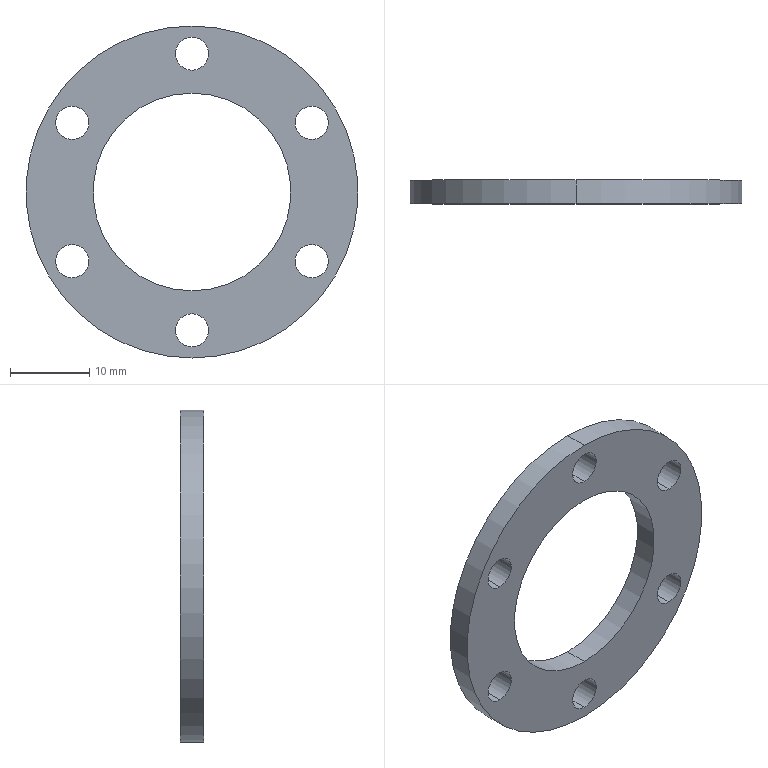Part | SolidWorks | features Extrusion 1 | 1 solid | 18 faces | box 42 x 3 x 42 mm | volume 2434 mm3 | cylinder 16 | plane 2 | commonest cylinder face diameters 4.2 x12 25 x2 42 x2
STEP:
#1=CARTESIAN_POINT('',(-15.155,3.,-10.85));
#2=VERTEX_POINT('',#1);
#3=CARTESIAN_POINT('',(-15.155,3.,-6.65));
#4=VERTEX_POINT('',#3);
#5=CARTESIAN_POINT('',(-15.155,3.,-8.75));
#6=DIRECTION('',(0.,1.,0.));
#7=DIRECTION('',(0.,0.,1.));
#8=AXIS2_PLACEMENT_3D('',#5,#6,#7);
#9=CIRCLE('',#8,2.1);
#10=EDGE_CURVE('',#2,#4,#9,.T.);
#11=ORIENTED_EDGE('',*,*,#10,.T.);
#12=CARTESIAN_POINT('',(-15.155,0.,-6.65));
#13=VERTEX_POINT('',#12);
#14=CARTESIAN_POINT('',(-15.155,3.,-6.65));
#15=DIRECTION('',(0.,-1.,0.));
#16=VECTOR('',#15,1000.);
#17=LINE('',#14,#16);
#18=EDGE_CURVE('',#4,#13,#17,.T.);
#19=ORIENTED_EDGE('',*,*,#18,.T.);
#20=CARTESIAN_POINT('',(-15.155,0.,-10.85));
#21=VERTEX_POINT('',#20);
#22=CARTESIAN_POINT('',(-15.155,0.,-8.75));
#23=DIRECTION('',(0.,1.,0.));
#24=DIRECTION('',(0.,0.,1.));
#25=AXIS2_PLACEMENT_3D('',#22,#23,#24);
#26=CIRCLE('',#25,2.1);
#27=EDGE_CURVE('',#21,#13,#26,.T.);
#28=ORIENTED_EDGE('',*,*,#27,.F.);
#29=CARTESIAN_POINT('',(-15.155,3.,-10.85));
#30=DIRECTION('',(0.,-1.,0.));
#31=VECTOR('',#30,1000.);
#32=LINE('',#29,#31);
#33=EDGE_CURVE('',#2,#21,#32,.T.);
#34=ORIENTED_EDGE('',*,*,#33,.F.);
#35=EDGE_LOOP('',(#11,#19,#28,#34));
#36=FACE_OUTER_BOUND('',#35,.T.);
#37=CARTESIAN_POINT('',(-15.155,3.,-8.75));
#38=DIRECTION('',(0.,-1.,0.));
#39=DIRECTION('',(0.,0.,-1.));
#40=AXIS2_PLACEMENT_3D('',#37,#38,#39);
#41=CYLINDRICAL_SURFACE('',#40,2.1);
#42=ADVANCED_FACE('',(#36),#41,.F.);
#43=CARTESIAN_POINT('',(-15.155,3.,6.65));
#44=VERTEX_POINT('',#43);
#45=CARTESIAN_POINT('',(-15.155,3.,10.85));
#46=VERTEX_POINT('',#45);
#47=CARTESIAN_POINT('',(-15.155,3.,8.75));
#48=DIRECTION('',(0.,1.,0.));
#49=DIRECTION('',(0.,0.,1.));
#50=AXIS2_PLACEMENT_3D('',#47,#48,#49);
#51=CIRCLE('',#50,2.1);
#52=EDGE_CURVE('',#44,#46,#51,.T.);
#53=ORIENTED_EDGE('',*,*,#52,.T.);
#54=CARTESIAN_POINT('',(-15.155,0.,10.85));
#55=VERTEX_POINT('',#54);
#56=CARTESIAN_POINT('',(-15.155,3.,10.85));
#57=DIRECTION('',(0.,-1.,0.));
#58=VECTOR('',#57,1000.);
#59=LINE('',#56,#58);
#60=EDGE_CURVE('',#46,#55,#59,.T.);
#61=ORIENTED_EDGE('',*,*,#60,.T.);
#62=CARTESIAN_POINT('',(-15.155,0.,6.65));
#63=VERTEX_POINT('',#62);
#64=CARTESIAN_POINT('',(-15.155,0.,8.75));
#65=DIRECTION('',(0.,1.,0.));
#66=DIRECTION('',(0.,0.,1.));
#67=AXIS2_PLACEMENT_3D('',#64,#65,#66);
#68=CIRCLE('',#67,2.1);
#69=EDGE_CURVE('',#63,#55,#68,.T.);
#70=ORIENTED_EDGE('',*,*,#69,.F.);
#71=CARTESIAN_POINT('',(-15.155,3.,6.65));
#72=DIRECTION('',(0.,-1.,0.));
#73=VECTOR('',#72,1000.);
#74=LINE('',#71,#73);
#75=EDGE_CURVE('',#44,#63,#74,.T.);
#76=ORIENTED_EDGE('',*,*,#75,.F.);
#77=EDGE_LOOP('',(#53,#61,#70,#76));
#78=FACE_OUTER_BOUND('',#77,.T.);
#79=CARTESIAN_POINT('',(-15.155,3.,8.75));
#80=DIRECTION('',(0.,-1.,0.));
#81=DIRECTION('',(0.,0.,-1.));
#82=AXIS2_PLACEMENT_3D('',#79,#80,#81);
#83=CYLINDRICAL_SURFACE('',#82,2.1);
#84=ADVANCED_FACE('',(#78),#83,.F.);
#85=CARTESIAN_POINT('',(0.,3.,15.4));
#86=VERTEX_POINT('',#85);
#87=CARTESIAN_POINT('',(0.,3.,19.6));
#88=VERTEX_POINT('',#87);
#89=CARTESIAN_POINT('',(0.,3.,17.5));
#90=DIRECTION('',(0.,1.,0.));
#91=DIRECTION('',(0.,0.,1.));
#92=AXIS2_PLACEMENT_3D('',#89,#90,#91);
#93=CIRCLE('',#92,2.1);
#94=EDGE_CURVE('',#86,#88,#93,.T.);
#95=ORIENTED_EDGE('',*,*,#94,.T.);
#96=CARTESIAN_POINT('',(0.,0.,19.6));
#97=VERTEX_POINT('',#96);
#98=CARTESIAN_POINT('',(0.,3.,19.6));
#99=DIRECTION('',(0.,-1.,0.));
#100=VECTOR('',#99,1000.);
#101=LINE('',#98,#100);
#102=EDGE_CURVE('',#88,#97,#101,.T.);
#103=ORIENTED_EDGE('',*,*,#102,.T.);
#104=CARTESIAN_POINT('',(0.,0.,15.4));
#105=VERTEX_POINT('',#104);
#106=CARTESIAN_POINT('',(0.,0.,17.5));
#107=DIRECTION('',(0.,1.,0.));
#108=DIRECTION('',(0.,0.,1.));
#109=AXIS2_PLACEMENT_3D('',#106,#107,#108);
#110=CIRCLE('',#109,2.1);
#111=EDGE_CURVE('',#105,#97,#110,.T.);
#112=ORIENTED_EDGE('',*,*,#111,.F.);
#113=CARTESIAN_POINT('',(0.,3.,15.4));
#114=DIRECTION('',(0.,-1.,0.));
#115=VECTOR('',#114,1000.);
#116=LINE('',#113,#115);
#117=EDGE_CURVE('',#86,#105,#116,.T.);
#118=ORIENTED_EDGE('',*,*,#117,.F.);
#119=EDGE_LOOP('',(#95,#103,#112,#118));
#120=FACE_OUTER_BOUND('',#119,.T.);
#121=CARTESIAN_POINT('',(0.,3.,17.5));
#122=DIRECTION('',(0.,-1.,0.));
#123=DIRECTION('',(0.,0.,-1.));
#124=AXIS2_PLACEMENT_3D('',#121,#122,#123);
#125=CYLINDRICAL_SURFACE('',#124,2.1);
#126=ADVANCED_FACE('',(#120),#125,.F.);
#127=CARTESIAN_POINT('',(15.155,3.,6.65));
#128=VERTEX_POINT('',#127);
#129=CARTESIAN_POINT('',(15.155,3.,10.85));
#130=VERTEX_POINT('',#129);
#131=CARTESIAN_POINT('',(15.155,3.,8.75));
#132=DIRECTION('',(0.,1.,0.));
#133=DIRECTION('',(0.,0.,1.));
#134=AXIS2_PLACEMENT_3D('',#131,#132,#133);
#135=CIRCLE('',#134,2.1);
#136=EDGE_CURVE('',#128,#130,#135,.T.);
#137=ORIENTED_EDGE('',*,*,#136,.T.);
#138=CARTESIAN_POINT('',(15.155,0.,10.85));
#139=VERTEX_POINT('',#138);
#140=CARTESIAN_POINT('',(15.155,3.,10.85));
#141=DIRECTION('',(0.,-1.,0.));
#142=VECTOR('',#141,1000.);
#143=LINE('',#140,#142);
#144=EDGE_CURVE('',#130,#139,#143,.T.);
#145=ORIENTED_EDGE('',*,*,#144,.T.);
#146=CARTESIAN_POINT('',(15.155,0.,6.65));
#147=VERTEX_POINT('',#146);
#148=CARTESIAN_POINT('',(15.155,0.,8.75));
#149=DIRECTION('',(0.,1.,0.));
#150=DIRECTION('',(0.,0.,1.));
#151=AXIS2_PLACEMENT_3D('',#148,#149,#150);
#152=CIRCLE('',#151,2.1);
#153=EDGE_CURVE('',#147,#139,#152,.T.);
#154=ORIENTED_EDGE('',*,*,#153,.F.);
#155=CARTESIAN_POINT('',(15.155,3.,6.65));
#156=DIRECTION('',(0.,-1.,0.));
#157=VECTOR('',#156,1000.);
#158=LINE('',#155,#157);
#159=EDGE_CURVE('',#128,#147,#158,.T.);
#160=ORIENTED_EDGE('',*,*,#159,.F.);
#161=EDGE_LOOP('',(#137,#145,#154,#160));
#162=FACE_OUTER_BOUND('',#161,.T.);
#163=CARTESIAN_POINT('',(15.155,3.,8.75));
#164=DIRECTION('',(0.,-1.,0.));
#165=DIRECTION('',(0.,0.,-1.));
#166=AXIS2_PLACEMENT_3D('',#163,#164,#165);
#167=CYLINDRICAL_SURFACE('',#166,2.1);
#168=ADVANCED_FACE('',(#162),#167,.F.);
#169=CARTESIAN_POINT('',(15.155,3.,-10.85));
#170=VERTEX_POINT('',#169);
#171=CARTESIAN_POINT('',(15.155,3.,-6.65));
#172=VERTEX_POINT('',#171);
#173=CARTESIAN_POINT('',(15.155,3.,-8.75));
#174=DIRECTION('',(0.,1.,0.));
#175=DIRECTION('',(0.,0.,1.));
#176=AXIS2_PLACEMENT_3D('',#173,#174,#175);
#177=CIRCLE('',#176,2.1);
#178=EDGE_CURVE('',#170,#172,#177,.T.);
#179=ORIENTED_EDGE('',*,*,#178,.T.);
#180=CARTESIAN_POINT('',(15.155,0.,-6.65));
#181=VERTEX_POINT('',#180);
#182=CARTESIAN_POINT('',(15.155,3.,-6.65));
#183=DIRECTION('',(0.,-1.,0.));
#184=VECTOR('',#183,1000.);
#185=LINE('',#182,#184);
#186=EDGE_CURVE('',#172,#181,#185,.T.);
#187=ORIENTED_EDGE('',*,*,#186,.T.);
#188=CARTESIAN_POINT('',(15.155,0.,-10.85));
#189=VERTEX_POINT('',#188);
#190=CARTESIAN_POINT('',(15.155,0.,-8.75));
#191=DIRECTION('',(0.,1.,0.));
#192=DIRECTION('',(0.,0.,1.));
#193=AXIS2_PLACEMENT_3D('',#190,#191,#192);
#194=CIRCLE('',#193,2.1);
#195=EDGE_CURVE('',#189,#181,#194,.T.);
#196=ORIENTED_EDGE('',*,*,#195,.F.);
#197=CARTESIAN_POINT('',(15.155,3.,-10.85));
#198=DIRECTION('',(0.,-1.,0.));
#199=VECTOR('',#198,1000.);
#200=LINE('',#197,#199);
#201=EDGE_CURVE('',#170,#189,#200,.T.);
#202=ORIENTED_EDGE('',*,*,#201,.F.);
#203=EDGE_LOOP('',(#179,#187,#196,#202));
#204=FACE_OUTER_BOUND('',#203,.T.);
#205=CARTESIAN_POINT('',(15.155,3.,-8.75));
#206=DIRECTION('',(0.,-1.,0.));
#207=DIRECTION('',(0.,0.,-1.));
#208=AXIS2_PLACEMENT_3D('',#205,#206,#207);
#209=CYLINDRICAL_SURFACE('',#208,2.1);
#210=ADVANCED_FACE('',(#204),#209,.F.);
#211=CARTESIAN_POINT('',(0.,3.,-19.6));
#212=VERTEX_POINT('',#211);
#213=CARTESIAN_POINT('',(0.,3.,-15.4));
#214=VERTEX_POINT('',#213);
#215=CARTESIAN_POINT('',(0.,3.,-17.5));
#216=DIRECTION('',(0.,1.,0.));
#217=DIRECTION('',(0.,0.,1.));
#218=AXIS2_PLACEMENT_3D('',#215,#216,#217);
#219=CIRCLE('',#218,2.1);
#220=EDGE_CURVE('',#212,#214,#219,.T.);
#221=ORIENTED_EDGE('',*,*,#220,.T.);
#222=CARTESIAN_POINT('',(0.,0.,-15.4));
#223=VERTEX_POINT('',#222);
#224=CARTESIAN_POINT('',(0.,3.,-15.4));
#225=DIRECTION('',(0.,-1.,0.));
#226=VECTOR('',#225,1000.);
#227=LINE('',#224,#226);
#228=EDGE_CURVE('',#214,#223,#227,.T.);
#229=ORIENTED_EDGE('',*,*,#228,.T.);
#230=CARTESIAN_POINT('',(0.,0.,-19.6));
#231=VERTEX_POINT('',#230);
#232=CARTESIAN_POINT('',(0.,0.,-17.5));
#233=DIRECTION('',(0.,1.,0.));
#234=DIRECTION('',(0.,0.,1.));
#235=AXIS2_PLACEMENT_3D('',#232,#233,#234);
#236=CIRCLE('',#235,2.1);
#237=EDGE_CURVE('',#231,#223,#236,.T.);
#238=ORIENTED_EDGE('',*,*,#237,.F.);
#239=CARTESIAN_POINT('',(0.,3.,-19.6));
#240=DIRECTION('',(0.,-1.,0.));
#241=VECTOR('',#240,1000.);
#242=LINE('',#239,#241);
#243=EDGE_CURVE('',#212,#231,#242,.T.);
#244=ORIENTED_EDGE('',*,*,#243,.F.);
#245=EDGE_LOOP('',(#221,#229,#238,#244));
#246=FACE_OUTER_BOUND('',#245,.T.);
#247=CARTESIAN_POINT('',(0.,3.,-17.5));
#248=DIRECTION('',(0.,-1.,0.));
#249=DIRECTION('',(0.,0.,-1.));
#250=AXIS2_PLACEMENT_3D('',#247,#248,#249);
#251=CYLINDRICAL_SURFACE('',#250,2.1);
#252=ADVANCED_FACE('',(#246),#251,.F.);
#253=CARTESIAN_POINT('',(0.,3.,-12.5));
#254=VERTEX_POINT('',#253);
#255=CARTESIAN_POINT('',(0.,3.,12.5));
#256=VERTEX_POINT('',#255);
#257=CARTESIAN_POINT('',(0.,3.,0.));
#258=DIRECTION('',(0.,1.,0.));
#259=DIRECTION('',(0.,0.,1.));
#260=AXIS2_PLACEMENT_3D('',#257,#258,#259);
#261=CIRCLE('',#260,12.5);
#262=EDGE_CURVE('',#254,#256,#261,.T.);
#263=ORIENTED_EDGE('',*,*,#262,.T.);
#264=CARTESIAN_POINT('',(0.,0.,12.5));
#265=VERTEX_POINT('',#264);
#266=CARTESIAN_POINT('',(0.,3.,12.5));
#267=DIRECTION('',(0.,-1.,0.));
#268=VECTOR('',#267,1000.);
#269=LINE('',#266,#268);
#270=EDGE_CURVE('',#256,#265,#269,.T.);
#271=ORIENTED_EDGE('',*,*,#270,.T.);
#272=CARTESIAN_POINT('',(0.,0.,-12.5));
#273=VERTEX_POINT('',#272);
#274=CARTESIAN_POINT('',(0.,0.,0.));
#275=DIRECTION('',(0.,1.,0.));
#276=DIRECTION('',(0.,0.,1.));
#277=AXIS2_PLACEMENT_3D('',#274,#275,#276);
#278=CIRCLE('',#277,12.5);
#279=EDGE_CURVE('',#273,#265,#278,.T.);
#280=ORIENTED_EDGE('',*,*,#279,.F.);
#281=CARTESIAN_POINT('',(0.,3.,-12.5));
#282=DIRECTION('',(0.,-1.,0.));
#283=VECTOR('',#282,1000.);
#284=LINE('',#281,#283);
#285=EDGE_CURVE('',#254,#273,#284,.T.);
#286=ORIENTED_EDGE('',*,*,#285,.F.);
#287=EDGE_LOOP('',(#263,#271,#280,#286));
#288=FACE_OUTER_BOUND('',#287,.T.);
#289=CARTESIAN_POINT('',(0.,3.,0.));
#290=DIRECTION('',(0.,-1.,0.));
#291=DIRECTION('',(0.,0.,-1.));
#292=AXIS2_PLACEMENT_3D('',#289,#290,#291);
#293=CYLINDRICAL_SURFACE('',#292,12.5);
#294=ADVANCED_FACE('',(#288),#293,.F.);
#295=CARTESIAN_POINT('',(0.,3.,21.));
#296=VERTEX_POINT('',#295);
#297=CARTESIAN_POINT('',(0.,3.,-21.));
#298=VERTEX_POINT('',#297);
#299=CARTESIAN_POINT('',(0.,3.,0.));
#300=DIRECTION('',(0.,1.,0.));
#301=DIRECTION('',(0.,0.,1.));
#302=AXIS2_PLACEMENT_3D('',#299,#300,#301);
#303=CIRCLE('',#302,21.);
#304=EDGE_CURVE('',#296,#298,#303,.T.);
#305=ORIENTED_EDGE('',*,*,#304,.F.);
#306=CARTESIAN_POINT('',(0.,0.,21.));
#307=VERTEX_POINT('',#306);
#308=CARTESIAN_POINT('',(0.,3.,21.));
#309=DIRECTION('',(0.,-1.,0.));
#310=VECTOR('',#309,1000.);
#311=LINE('',#308,#310);
#312=EDGE_CURVE('',#296,#307,#311,.T.);
#313=ORIENTED_EDGE('',*,*,#312,.T.);
#314=CARTESIAN_POINT('',(0.,0.,-21.));
#315=VERTEX_POINT('',#314);
#316=CARTESIAN_POINT('',(0.,0.,0.));
#317=DIRECTION('',(0.,1.,0.));
#318=DIRECTION('',(0.,0.,1.));
#319=AXIS2_PLACEMENT_3D('',#316,#317,#318);
#320=CIRCLE('',#319,21.);
#321=EDGE_CURVE('',#307,#315,#320,.T.);
#322=ORIENTED_EDGE('',*,*,#321,.T.);
#323=CARTESIAN_POINT('',(0.,3.,-21.));
#324=DIRECTION('',(0.,-1.,0.));
#325=VECTOR('',#324,1000.);
#326=LINE('',#323,#325);
#327=EDGE_CURVE('',#298,#315,#326,.T.);
#328=ORIENTED_EDGE('',*,*,#327,.F.);
#329=EDGE_LOOP('',(#305,#313,#322,#328));
#330=FACE_OUTER_BOUND('',#329,.T.);
#331=CARTESIAN_POINT('',(0.,3.,0.));
#332=DIRECTION('',(0.,-1.,0.));
#333=DIRECTION('',(0.,0.,-1.));
#334=AXIS2_PLACEMENT_3D('',#331,#332,#333);
#335=CYLINDRICAL_SURFACE('',#334,21.);
#336=ADVANCED_FACE('',(#330),#335,.T.);
#337=ORIENTED_EDGE('',*,*,#52,.F.);
#338=CARTESIAN_POINT('',(-15.155,3.,8.75));
#339=DIRECTION('',(0.,1.,0.));
#340=DIRECTION('',(0.,0.,1.));
#341=AXIS2_PLACEMENT_3D('',#338,#339,#340);
#342=CIRCLE('',#341,2.1);
#343=EDGE_CURVE('',#46,#44,#342,.T.);
#344=ORIENTED_EDGE('',*,*,#343,.F.);
#345=EDGE_LOOP('',(#337,#344));
#346=FACE_BOUND('',#345,.T.);
#347=ORIENTED_EDGE('',*,*,#136,.F.);
#348=CARTESIAN_POINT('',(15.155,3.,8.75));
#349=DIRECTION('',(0.,1.,0.));
#350=DIRECTION('',(0.,0.,1.));
#351=AXIS2_PLACEMENT_3D('',#348,#349,#350);
#352=CIRCLE('',#351,2.1);
#353=EDGE_CURVE('',#130,#128,#352,.T.);
#354=ORIENTED_EDGE('',*,*,#353,.F.);
#355=EDGE_LOOP('',(#347,#354));
#356=FACE_BOUND('',#355,.T.);
#357=ORIENTED_EDGE('',*,*,#220,.F.);
#358=CARTESIAN_POINT('',(0.,3.,-17.5));
#359=DIRECTION('',(0.,1.,0.));
#360=DIRECTION('',(0.,0.,1.));
#361=AXIS2_PLACEMENT_3D('',#358,#359,#360);
#362=CIRCLE('',#361,2.1);
#363=EDGE_CURVE('',#214,#212,#362,.T.);
#364=ORIENTED_EDGE('',*,*,#363,.F.);
#365=EDGE_LOOP('',(#357,#364));
#366=FACE_BOUND('',#365,.T.);
#367=CARTESIAN_POINT('',(0.,3.,0.));
#368=DIRECTION('',(0.,1.,0.));
#369=DIRECTION('',(0.,0.,1.));
#370=AXIS2_PLACEMENT_3D('',#367,#368,#369);
#371=CIRCLE('',#370,21.);
#372=EDGE_CURVE('',#298,#296,#371,.T.);
#373=ORIENTED_EDGE('',*,*,#372,.T.);
#374=ORIENTED_EDGE('',*,*,#304,.T.);
#375=EDGE_LOOP('',(#373,#374));
#376=FACE_OUTER_BOUND('',#375,.T.);
#377=ORIENTED_EDGE('',*,*,#262,.F.);
#378=CARTESIAN_POINT('',(0.,3.,0.));
#379=DIRECTION('',(0.,1.,0.));
#380=DIRECTION('',(0.,0.,1.));
#381=AXIS2_PLACEMENT_3D('',#378,#379,#380);
#382=CIRCLE('',#381,12.5);
#383=EDGE_CURVE('',#256,#254,#382,.T.);
#384=ORIENTED_EDGE('',*,*,#383,.F.);
#385=EDGE_LOOP('',(#377,#384));
#386=FACE_BOUND('',#385,.T.);
#387=ORIENTED_EDGE('',*,*,#178,.F.);
#388=CARTESIAN_POINT('',(15.155,3.,-8.75));
#389=DIRECTION('',(0.,1.,0.));
#390=DIRECTION('',(0.,0.,1.));
#391=AXIS2_PLACEMENT_3D('',#388,#389,#390);
#392=CIRCLE('',#391,2.1);
#393=EDGE_CURVE('',#172,#170,#392,.T.);
#394=ORIENTED_EDGE('',*,*,#393,.F.);
#395=EDGE_LOOP('',(#387,#394));
#396=FACE_BOUND('',#395,.T.);
#397=ORIENTED_EDGE('',*,*,#94,.F.);
#398=CARTESIAN_POINT('',(0.,3.,17.5));
#399=DIRECTION('',(0.,1.,0.));
#400=DIRECTION('',(0.,0.,1.));
#401=AXIS2_PLACEMENT_3D('',#398,#399,#400);
#402=CIRCLE('',#401,2.1);
#403=EDGE_CURVE('',#88,#86,#402,.T.);
#404=ORIENTED_EDGE('',*,*,#403,.F.);
#405=EDGE_LOOP('',(#397,#404));
#406=FACE_BOUND('',#405,.T.);
#407=ORIENTED_EDGE('',*,*,#10,.F.);
#408=CARTESIAN_POINT('',(-15.155,3.,-8.75));
#409=DIRECTION('',(0.,1.,0.));
#410=DIRECTION('',(0.,0.,1.));
#411=AXIS2_PLACEMENT_3D('',#408,#409,#410);
#412=CIRCLE('',#411,2.1);
#413=EDGE_CURVE('',#4,#2,#412,.T.);
#414=ORIENTED_EDGE('',*,*,#413,.F.);
#415=EDGE_LOOP('',(#407,#414));
#416=FACE_BOUND('',#415,.T.);
#417=CARTESIAN_POINT('',(0.,3.,0.));
#418=DIRECTION('',(0.,1.,0.));
#419=DIRECTION('',(0.,0.,1.));
#420=AXIS2_PLACEMENT_3D('',#417,#418,#419);
#421=PLANE('',#420);
#422=ADVANCED_FACE('',(#346,#356,#366,#376,#386,#396,#406,#416),#421,.T.);
#423=CARTESIAN_POINT('',(0.,0.,0.));
#424=DIRECTION('',(0.,1.,0.));
#425=DIRECTION('',(0.,0.,1.));
#426=AXIS2_PLACEMENT_3D('',#423,#424,#425);
#427=CIRCLE('',#426,21.);
#428=EDGE_CURVE('',#315,#307,#427,.T.);
#429=ORIENTED_EDGE('',*,*,#428,.F.);
#430=ORIENTED_EDGE('',*,*,#321,.F.);
#431=EDGE_LOOP('',(#429,#430));
#432=FACE_OUTER_BOUND('',#431,.T.);
#433=ORIENTED_EDGE('',*,*,#279,.T.);
#434=CARTESIAN_POINT('',(0.,0.,0.));
#435=DIRECTION('',(0.,1.,0.));
#436=DIRECTION('',(0.,0.,1.));
#437=AXIS2_PLACEMENT_3D('',#434,#435,#436);
#438=CIRCLE('',#437,12.5);
#439=EDGE_CURVE('',#265,#273,#438,.T.);
#440=ORIENTED_EDGE('',*,*,#439,.T.);
#441=EDGE_LOOP('',(#433,#440));
#442=FACE_BOUND('',#441,.T.);
#443=ORIENTED_EDGE('',*,*,#237,.T.);
#444=CARTESIAN_POINT('',(0.,0.,-17.5));
#445=DIRECTION('',(0.,1.,0.));
#446=DIRECTION('',(0.,0.,1.));
#447=AXIS2_PLACEMENT_3D('',#444,#445,#446);
#448=CIRCLE('',#447,2.1);
#449=EDGE_CURVE('',#223,#231,#448,.T.);
#450=ORIENTED_EDGE('',*,*,#449,.T.);
#451=EDGE_LOOP('',(#443,#450));
#452=FACE_BOUND('',#451,.T.);
#453=ORIENTED_EDGE('',*,*,#195,.T.);
#454=CARTESIAN_POINT('',(15.155,0.,-8.75));
#455=DIRECTION('',(0.,1.,0.));
#456=DIRECTION('',(0.,0.,1.));
#457=AXIS2_PLACEMENT_3D('',#454,#455,#456);
#458=CIRCLE('',#457,2.1);
#459=EDGE_CURVE('',#181,#189,#458,.T.);
#460=ORIENTED_EDGE('',*,*,#459,.T.);
#461=EDGE_LOOP('',(#453,#460));
#462=FACE_BOUND('',#461,.T.);
#463=ORIENTED_EDGE('',*,*,#153,.T.);
#464=CARTESIAN_POINT('',(15.155,0.,8.75));
#465=DIRECTION('',(0.,1.,0.));
#466=DIRECTION('',(0.,0.,1.));
#467=AXIS2_PLACEMENT_3D('',#464,#465,#466);
#468=CIRCLE('',#467,2.1);
#469=EDGE_CURVE('',#139,#147,#468,.T.);
#470=ORIENTED_EDGE('',*,*,#469,.T.);
#471=EDGE_LOOP('',(#463,#470));
#472=FACE_BOUND('',#471,.T.);
#473=ORIENTED_EDGE('',*,*,#111,.T.);
#474=CARTESIAN_POINT('',(0.,0.,17.5));
#475=DIRECTION('',(0.,1.,0.));
#476=DIRECTION('',(0.,0.,1.));
#477=AXIS2_PLACEMENT_3D('',#474,#475,#476);
#478=CIRCLE('',#477,2.1);
#479=EDGE_CURVE('',#97,#105,#478,.T.);
#480=ORIENTED_EDGE('',*,*,#479,.T.);
#481=EDGE_LOOP('',(#473,#480));
#482=FACE_BOUND('',#481,.T.);
#483=ORIENTED_EDGE('',*,*,#69,.T.);
#484=CARTESIAN_POINT('',(-15.155,0.,8.75));
#485=DIRECTION('',(0.,1.,0.));
#486=DIRECTION('',(0.,0.,1.));
#487=AXIS2_PLACEMENT_3D('',#484,#485,#486);
#488=CIRCLE('',#487,2.1);
#489=EDGE_CURVE('',#55,#63,#488,.T.);
#490=ORIENTED_EDGE('',*,*,#489,.T.);
#491=EDGE_LOOP('',(#483,#490));
#492=FACE_BOUND('',#491,.T.);
#493=ORIENTED_EDGE('',*,*,#27,.T.);
#494=CARTESIAN_POINT('',(-15.155,0.,-8.75));
#495=DIRECTION('',(0.,1.,0.));
#496=DIRECTION('',(0.,0.,1.));
#497=AXIS2_PLACEMENT_3D('',#494,#495,#496);
#498=CIRCLE('',#497,2.1);
#499=EDGE_CURVE('',#13,#21,#498,.T.);
#500=ORIENTED_EDGE('',*,*,#499,.T.);
#501=EDGE_LOOP('',(#493,#500));
#502=FACE_BOUND('',#501,.T.);
#503=CARTESIAN_POINT('',(0.,0.,0.));
#504=DIRECTION('',(0.,1.,0.));
#505=DIRECTION('',(0.,0.,1.));
#506=AXIS2_PLACEMENT_3D('',#503,#504,#505);
#507=PLANE('',#506);
#508=ADVANCED_FACE('',(#432,#442,#452,#462,#472,#482,#492,#502),#507,.F.);
#509=ORIENTED_EDGE('',*,*,#312,.F.);
#510=ORIENTED_EDGE('',*,*,#372,.F.);
#511=ORIENTED_EDGE('',*,*,#327,.T.);
#512=ORIENTED_EDGE('',*,*,#428,.T.);
#513=EDGE_LOOP('',(#509,#510,#511,#512));
#514=FACE_OUTER_BOUND('',#513,.T.);
#515=CARTESIAN_POINT('',(0.,3.,0.));
#516=DIRECTION('',(0.,-1.,0.));
#517=DIRECTION('',(0.,0.,-1.));
#518=AXIS2_PLACEMENT_3D('',#515,#516,#517);
#519=CYLINDRICAL_SURFACE('',#518,21.);
#520=ADVANCED_FACE('',(#514),#519,.T.);
#521=ORIENTED_EDGE('',*,*,#270,.F.);
#522=ORIENTED_EDGE('',*,*,#383,.T.);
#523=ORIENTED_EDGE('',*,*,#285,.T.);
#524=ORIENTED_EDGE('',*,*,#439,.F.);
#525=EDGE_LOOP('',(#521,#522,#523,#524));
#526=FACE_OUTER_BOUND('',#525,.T.);
#527=CARTESIAN_POINT('',(0.,3.,0.));
#528=DIRECTION('',(0.,-1.,0.));
#529=DIRECTION('',(0.,0.,-1.));
#530=AXIS2_PLACEMENT_3D('',#527,#528,#529);
#531=CYLINDRICAL_SURFACE('',#530,12.5);
#532=ADVANCED_FACE('',(#526),#531,.F.);
#533=ORIENTED_EDGE('',*,*,#228,.F.);
#534=ORIENTED_EDGE('',*,*,#363,.T.);
#535=ORIENTED_EDGE('',*,*,#243,.T.);
#536=ORIENTED_EDGE('',*,*,#449,.F.);
#537=EDGE_LOOP('',(#533,#534,#535,#536));
#538=FACE_OUTER_BOUND('',#537,.T.);
#539=CARTESIAN_POINT('',(0.,3.,-17.5));
#540=DIRECTION('',(0.,-1.,0.));
#541=DIRECTION('',(0.,0.,-1.));
#542=AXIS2_PLACEMENT_3D('',#539,#540,#541);
#543=CYLINDRICAL_SURFACE('',#542,2.1);
#544=ADVANCED_FACE('',(#538),#543,.F.);
#545=ORIENTED_EDGE('',*,*,#186,.F.);
#546=ORIENTED_EDGE('',*,*,#393,.T.);
#547=ORIENTED_EDGE('',*,*,#201,.T.);
#548=ORIENTED_EDGE('',*,*,#459,.F.);
#549=EDGE_LOOP('',(#545,#546,#547,#548));
#550=FACE_OUTER_BOUND('',#549,.T.);
#551=CARTESIAN_POINT('',(15.155,3.,-8.75));
#552=DIRECTION('',(0.,-1.,0.));
#553=DIRECTION('',(0.,0.,-1.));
#554=AXIS2_PLACEMENT_3D('',#551,#552,#553);
#555=CYLINDRICAL_SURFACE('',#554,2.1);
#556=ADVANCED_FACE('',(#550),#555,.F.);
#557=ORIENTED_EDGE('',*,*,#144,.F.);
#558=ORIENTED_EDGE('',*,*,#353,.T.);
#559=ORIENTED_EDGE('',*,*,#159,.T.);
#560=ORIENTED_EDGE('',*,*,#469,.F.);
#561=EDGE_LOOP('',(#557,#558,#559,#560));
#562=FACE_OUTER_BOUND('',#561,.T.);
#563=CARTESIAN_POINT('',(15.155,3.,8.75));
#564=DIRECTION('',(0.,-1.,0.));
#565=DIRECTION('',(0.,0.,-1.));
#566=AXIS2_PLACEMENT_3D('',#563,#564,#565);
#567=CYLINDRICAL_SURFACE('',#566,2.1);
#568=ADVANCED_FACE('',(#562),#567,.F.);
#569=ORIENTED_EDGE('',*,*,#102,.F.);
#570=ORIENTED_EDGE('',*,*,#403,.T.);
#571=ORIENTED_EDGE('',*,*,#117,.T.);
#572=ORIENTED_EDGE('',*,*,#479,.F.);
#573=EDGE_LOOP('',(#569,#570,#571,#572));
#574=FACE_OUTER_BOUND('',#573,.T.);
#575=CARTESIAN_POINT('',(0.,3.,17.5));
#576=DIRECTION('',(0.,-1.,0.));
#577=DIRECTION('',(0.,0.,-1.));
#578=AXIS2_PLACEMENT_3D('',#575,#576,#577);
#579=CYLINDRICAL_SURFACE('',#578,2.1);
#580=ADVANCED_FACE('',(#574),#579,.F.);
#581=ORIENTED_EDGE('',*,*,#60,.F.);
#582=ORIENTED_EDGE('',*,*,#343,.T.);
#583=ORIENTED_EDGE('',*,*,#75,.T.);
#584=ORIENTED_EDGE('',*,*,#489,.F.);
#585=EDGE_LOOP('',(#581,#582,#583,#584));
#586=FACE_OUTER_BOUND('',#585,.T.);
#587=CARTESIAN_POINT('',(-15.155,3.,8.75));
#588=DIRECTION('',(0.,-1.,0.));
#589=DIRECTION('',(0.,0.,-1.));
#590=AXIS2_PLACEMENT_3D('',#587,#588,#589);
#591=CYLINDRICAL_SURFACE('',#590,2.1);
#592=ADVANCED_FACE('',(#586),#591,.F.);
#593=ORIENTED_EDGE('',*,*,#18,.F.);
#594=ORIENTED_EDGE('',*,*,#413,.T.);
#595=ORIENTED_EDGE('',*,*,#33,.T.);
#596=ORIENTED_EDGE('',*,*,#499,.F.);
#597=EDGE_LOOP('',(#593,#594,#595,#596));
#598=FACE_OUTER_BOUND('',#597,.T.);
#599=CARTESIAN_POINT('',(-15.155,3.,-8.75));
#600=DIRECTION('',(0.,-1.,0.));
#601=DIRECTION('',(0.,0.,-1.));
#602=AXIS2_PLACEMENT_3D('',#599,#600,#601);
#603=CYLINDRICAL_SURFACE('',#602,2.1);
#604=ADVANCED_FACE('',(#598),#603,.F.);
#605=CLOSED_SHELL('',(#42,#84,#126,#168,#210,#252,#294,#336,#422,#508,#520,#532,#544,#556,#568,#580,#592,#604));
#606=MANIFOLD_SOLID_BREP('',#605);
#607=CARTESIAN_POINT('',(0.,0.,0.));
#608=DIRECTION('',(0.,0.,1.));
#609=DIRECTION('',(1.,0.,0.));
#610=AXIS2_PLACEMENT_3D('',#607,#608,#609);
#611=(LENGTH_UNIT()NAMED_UNIT(*)SI_UNIT(.MILLI.,.METRE.));
#612=UNCERTAINTY_MEASURE_WITH_UNIT(LENGTH_MEASURE(0.00001),#611,'','');
#613=(NAMED_UNIT(*)PLANE_ANGLE_UNIT()SI_UNIT($,.RADIAN.));
#614=(NAMED_UNIT(*)SI_UNIT($,.STERADIAN.)SOLID_ANGLE_UNIT());
#615=(GEOMETRIC_REPRESENTATION_CONTEXT(3)GLOBAL_UNCERTAINTY_ASSIGNED_CONTEXT((#612))GLOBAL_UNIT_ASSIGNED_CONTEXT((#611,#613,#614))REPRESENTATION_CONTEXT('',''));
#616=ADVANCED_BREP_SHAPE_REPRESENTATION('',(#606,#610),#615);